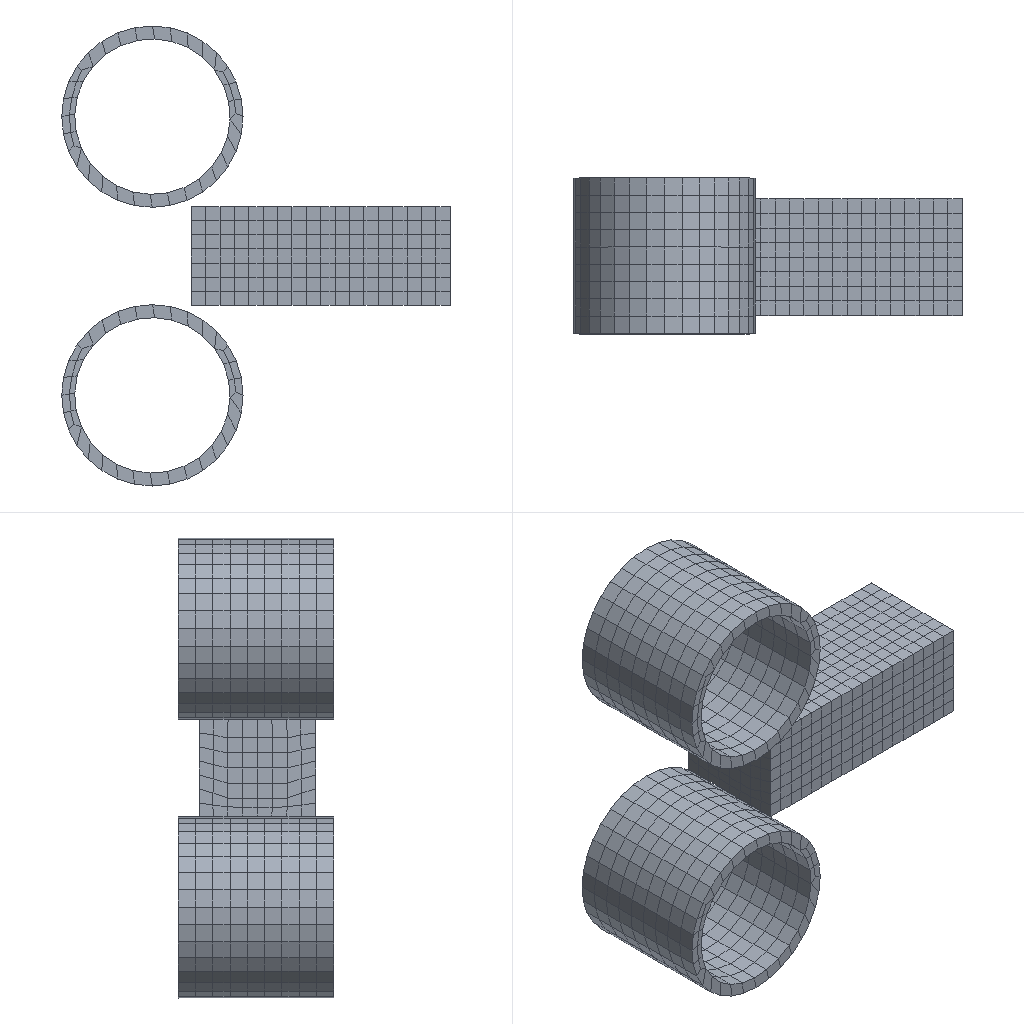Simulation study | abaqus
Set-up summary:
category,name,step,type,value,unit,region
solver,abaqus
solver,version,,,Abaqus/Explicit 2020
units,not stated in the deck,,not stated
analysis,deck,,dynamic temperature-displacement,dynamic temperature-displacement
load_step,Step-1,Step-1,dynamic temperature-displacement
load_step,requested,,,1
mesh,nodes,,,2768
mesh,elements,,,1728
element_type,C3D8R,,solid,720
element_type,C3D8RT,,solid,1008
load,load commands in deck,,count,3
bc,support commands in deck,,count,7
material,GUNZI,,in results
material,WORK,,in results
check,setup vs results,,match,"per instance, exact: element labels, types and connectivity; labels of the nodes the elements use; coordinates not compared"
Abaqus input file, long lists of numbers shortened:
*Heading
** Job name: Job-2 Model name: Model-1-Copy
** Generated by: Abaqus/CAE 2020
*Preprint, echo=NO, model=NO, history=NO, contact=NO
**
** PARTS
**
*Part, name=Part-1
*Node
      1,        1000.,  -108.96,   306.04
      2,        1000.,  -341.04,   306.04
** (1366 more lines like these left out)
*Element, type=C3D8RT
  1,   58,  349,  927,  247,    1,   17,  229,   28
  2,  349,  350,  928,  927,   17,   18,  230,  229
** (1006 more lines like these left out)
*Nset, nset=Set-6, generate
    1,  1368,     1
*Elset, elset=Set-6, generate
    1,  1008,     1
** Section: Section-1
*Solid Section, elset=Set-6, material=work
,
*End Part
**
*Part, name=gun
*Node
      1,   228.892,  -193.929,           0.
      2,   266.306,  -138.133,           0.
** (698 more lines like these left out)
*Element, type=C3D8R
  1, 107,  80,  81, 108,  37,  10,  11,  38
  2, 109, 108,  81,  82,  39,  38,  11,  12
** (358 more lines like these left out)
*Nset, nset=Set-3, generate
   1,  700,    1
*Elset, elset=Set-3, generate
   1,  360,    1
** Section: Section-2
*Solid Section, elset=Set-3, material=gunzi
,
*End Part
**
**
** ASSEMBLY
**
*Assembly, name=Assembly
**
*Instance, name=Part-1-1, part=Part-1
        150.,         -80.,        -728.
*End Instance
**
*Instance, name=gun-1, part=gun
          0.,           0.,           0.
          0.,           0.,           0., 1.,           0.,           0., 90.
*End Instance
**
*Instance, name=gun-1-lin-2-1, part=gun
          0.,           0.,       -1076.
          0.,           0.,       -1076., 1.,           0.,       -1076., 90.
*End Instance
**
*Node
      1,           0.,        -300.,       -1076.
*Node
      2,           0.,        -300., 1.83697018e-14
*Nset, nset=Set-3, instance=Part-1-1, generate
    1,  1368,     1
*Elset, elset=Set-3, instance=Part-1-1, generate
    1,  1008,     1
*Nset, nset=Set-4, instance=Part-1-1, generate
    1,  1368,     1
*Elset, elset=Set-4, instance=Part-1-1, generate
    1,  1008,     1
*Nset, nset=Set-9
 1, 2
*Nset, nset=Set-11, instance=Part-1-1, generate
    1,  1368,     1
*Elset, elset=Set-11, instance=Part-1-1, generate
    1,  1008,     1
*Nset, nset=Set-12, instance=Part-1-1, generate
    1,  1368,     1
*Elset, elset=Set-12, instance=Part-1-1, generate
    1,  1008,     1
*Nset, nset=Set-13, instance=Part-1-1
   1,   2,   3,   4,  17,  18,  19,  20,  21,  22,  23,  24,  25,  26,  27,  28
 229, 230, 231, 232, 233, 234, 235, 236, 237
*Elset, elset=Set-13, instance=Part-1-1, generate
  1,  16,   1
*Nset, nset=Set-14, instance=Part-1-1
   5,   6,   7,   8,   9,  10,  11,  12,  13,  14,  15,  16,  29,  30,  31,  32
  33,  34,  35,  36,  37,  38,  39,  40, 116, 117, 118, 119, 120, 121, 129, 130
** (21 more lines like these left out)
*Elset, elset=Set-14, instance=Part-1-1
  273,  274,  275,  276,  277,  278,  279,  280,  281,  282,  283,  284,  285,  286,  287,  288
  289,  298,  300,  301,  306,  308,  309,  310,  311,  312,  319,  321,  323,  325,  329,  338
** (17 more lines like these left out)
*Nset, nset=Set-15, instance=Part-1-1
   5,   6,   7,   8,  29,  30,  31,  32,  33,  34,  35,  36,  37,  38,  39,  40
 238, 239, 240, 241, 242, 243, 244, 245, 246
*Elset, elset=Set-15, instance=Part-1-1, generate
 273,  288,    1
*Nset, nset=Set-16, instance=Part-1-1
   5,   6,   7,   8,  29,  30,  31,  32,  33,  34,  35,  36,  37,  38,  39,  40
 238, 239, 240, 241, 242, 243, 244, 245, 246
*Elset, elset=Set-16, instance=Part-1-1, generate
 273,  288,    1
*Nset, nset=Set-17, instance=gun-1, generate
   1,  700,    1
*Nset, nset=Set-17, instance=gun-1-lin-2-1, generate
   1,  700,    1
*Elset, elset=Set-17, instance=gun-1, generate
   1,  360,    1
*Elset, elset=Set-17, instance=gun-1-lin-2-1, generate
   1,  360,    1
*Nset, nset=b_Set-5, instance=gun-1-lin-2-1, generate
   1,  700,    1
*Elset, elset=b_Set-5, instance=gun-1-lin-2-1, generate
   1,  360,    1
*Nset, nset=b_Set-7, instance=gun-1, generate
   1,  700,    1
*Elset, elset=b_Set-7, instance=gun-1, generate
   1,  360,    1
*Nset, nset=_PickedSet44, internal
 1,
*Nset, nset=_PickedSet46, internal
 2,
*Elset, elset=_Surf-18_S6, internal, instance=Part-1-1
  294,  300,  301,  303,  306,  308,  309,  310,  311,  312,  313,  314,  316,  322,  323,  328
  334,  340,  341,  343,  346,  348,  349,  350,  351,  352,  353,  354,  356,  362,  363,  368
** (16 more lines like these left out)
*Elset, elset=_Surf-18_S4, internal, instance=Part-1-1
  307,  318,  325,  347,  358,  365,  387,  398,  405,  427,  438,  445,  467,  478,  485,  507
  518,  525,  547,  558,  565,  587,  598,  605,  627,  638,  645,  667,  678,  685,  707,  718
** (2 more lines like these left out)
*Elset, elset=_Surf-18_S2, internal, instance=Part-1-1, generate
  969,  1008,     1
*Elset, elset=_Surf-18_S1, internal, instance=Part-1-1, generate
 273,  288,    1
*Elset, elset=_Surf-18_S3, internal, instance=Part-1-1
  289,  295,  297,  298,  301,  306,  319,  321,  329,  335,  337,  338,  341,  346,  359,  361
  369,  375,  377,  378,  381,  386,  399,  401,  409,  415,  417,  418,  421,  426,  439,  441
** (7 more lines like these left out)
*Elset, elset=_Surf-18_S5, internal, instance=Part-1-1
  308,  323,  327,  348,  363,  367,  388,  403,  407,  428,  443,  447,  468,  483,  487,  508
  523,  527,  548,  563,  567,  588,  603,  607,  628,  643,  647,  668,  683,  687,  708,  723
** (2 more lines like these left out)
*Surface, type=ELEMENT, name=Surf-18
_Surf-18_S6, S6
_Surf-18_S4, S4
_Surf-18_S2, S2
_Surf-18_S1, S1
_Surf-18_S3, S3
_Surf-18_S5, S5
*Elset, elset=_Surf-19_S6, internal, instance=Part-1-1
  294,  300,  301,  303,  306,  308,  309,  310,  311,  312,  313,  314,  316,  322,  323,  328
  334,  340,  341,  343,  346,  348,  349,  350,  351,  352,  353,  354,  356,  362,  363,  368
** (16 more lines like these left out)
*Elset, elset=_Surf-19_S4, internal, instance=Part-1-1
  307,  318,  325,  347,  358,  365,  387,  398,  405,  427,  438,  445,  467,  478,  485,  507
  518,  525,  547,  558,  565,  587,  598,  605,  627,  638,  645,  667,  678,  685,  707,  718
** (2 more lines like these left out)
*Elset, elset=_Surf-19_S2, internal, instance=Part-1-1, generate
  969,  1008,     1
*Elset, elset=_Surf-19_S1, internal, instance=Part-1-1, generate
 273,  288,    1
*Elset, elset=_Surf-19_S3, internal, instance=Part-1-1
  289,  295,  297,  298,  301,  306,  319,  321,  329,  335,  337,  338,  341,  346,  359,  361
  369,  375,  377,  378,  381,  386,  399,  401,  409,  415,  417,  418,  421,  426,  439,  441
** (7 more lines like these left out)
*Elset, elset=_Surf-19_S5, internal, instance=Part-1-1
  308,  323,  327,  348,  363,  367,  388,  403,  407,  428,  443,  447,  468,  483,  487,  508
  523,  527,  548,  563,  567,  588,  603,  607,  628,  643,  647,  668,  683,  687,  708,  723
** (2 more lines like these left out)
*Surface, type=ELEMENT, name=Surf-19
_Surf-19_S6, S6
_Surf-19_S4, S4
_Surf-19_S2, S2
_Surf-19_S1, S1
_Surf-19_S3, S3
_Surf-19_S5, S5
*Elset, elset=_Surf-20_S6, internal, instance=Part-1-1
  294,  300,  301,  303,  306,  308,  309,  310,  311,  312,  313,  314,  316,  322,  323,  328
  334,  340,  341,  343,  346,  348,  349,  350,  351,  352,  353,  354,  356,  362,  363,  368
** (16 more lines like these left out)
*Elset, elset=_Surf-20_S4, internal, instance=Part-1-1
  307,  318,  325,  347,  358,  365,  387,  398,  405,  427,  438,  445,  467,  478,  485,  507
  518,  525,  547,  558,  565,  587,  598,  605,  627,  638,  645,  667,  678,  685,  707,  718
** (2 more lines like these left out)
*Elset, elset=_Surf-20_S2, internal, instance=Part-1-1, generate
  969,  1008,     1
*Elset, elset=_Surf-20_S1, internal, instance=Part-1-1, generate
 273,  288,    1
*Elset, elset=_Surf-20_S3, internal, instance=Part-1-1
  289,  295,  297,  298,  301,  306,  319,  321,  329,  335,  337,  338,  341,  346,  359,  361
  369,  375,  377,  378,  381,  386,  399,  401,  409,  415,  417,  418,  421,  426,  439,  441
** (7 more lines like these left out)
*Elset, elset=_Surf-20_S5, internal, instance=Part-1-1
  308,  323,  327,  348,  363,  367,  388,  403,  407,  428,  443,  447,  468,  483,  487,  508
  523,  527,  548,  563,  567,  588,  603,  607,  628,  643,  647,  668,  683,  687,  708,  723
** (2 more lines like these left out)
*Surface, type=ELEMENT, name=Surf-20
_Surf-20_S6, S6
_Surf-20_S4, S4
_Surf-20_S2, S2
_Surf-20_S1, S1
_Surf-20_S3, S3
_Surf-20_S5, S5
*Elset, elset=_Surf-21_S6, internal, instance=Part-1-1
  294,  300,  301,  303,  306,  308,  309,  310,  311,  312,  313,  314,  316,  322,  323,  328
  334,  340,  341,  343,  346,  348,  349,  350,  351,  352,  353,  354,  356,  362,  363,  368
** (16 more lines like these left out)
*Elset, elset=_Surf-21_S4, internal, instance=Part-1-1
  307,  318,  325,  347,  358,  365,  387,  398,  405,  427,  438,  445,  467,  478,  485,  507
  518,  525,  547,  558,  565,  587,  598,  605,  627,  638,  645,  667,  678,  685,  707,  718
** (2 more lines like these left out)
*Elset, elset=_Surf-21_S2, internal, instance=Part-1-1, generate
  969,  1008,     1
*Elset, elset=_Surf-21_S1, internal, instance=Part-1-1, generate
 273,  288,    1
*Elset, elset=_Surf-21_S3, internal, instance=Part-1-1
  289,  295,  297,  298,  301,  306,  319,  321,  329,  335,  337,  338,  341,  346,  359,  361
  369,  375,  377,  378,  381,  386,  399,  401,  409,  415,  417,  418,  421,  426,  439,  441
** (7 more lines like these left out)
*Elset, elset=_Surf-21_S5, internal, instance=Part-1-1
  308,  323,  327,  348,  363,  367,  388,  403,  407,  428,  443,  447,  468,  483,  487,  508
  523,  527,  548,  563,  567,  588,  603,  607,  628,  643,  647,  668,  683,  687,  708,  723
** (2 more lines like these left out)
*Surface, type=ELEMENT, name=Surf-21
_Surf-21_S6, S6
_Surf-21_S4, S4
_Surf-21_S2, S2
_Surf-21_S1, S1
_Surf-21_S3, S3
_Surf-21_S5, S5
*Elset, elset=_Surf-22_S6, internal, instance=Part-1-1
  294,  300,  301,  303,  306,  308,  309,  310,  311,  312,  313,  314,  316,  322,  323,  328
  334,  340,  341,  343,  346,  348,  349,  350,  351,  352,  353,  354,  356,  362,  363,  368
** (16 more lines like these left out)
*Elset, elset=_Surf-22_S4, internal, instance=Part-1-1
  307,  318,  325,  347,  358,  365,  387,  398,  405,  427,  438,  445,  467,  478,  485,  507
  518,  525,  547,  558,  565,  587,  598,  605,  627,  638,  645,  667,  678,  685,  707,  718
** (2 more lines like these left out)
*Elset, elset=_Surf-22_S2, internal, instance=Part-1-1, generate
  969,  1008,     1
*Elset, elset=_Surf-22_S1, internal, instance=Part-1-1, generate
 273,  288,    1
*Elset, elset=_Surf-22_S3, internal, instance=Part-1-1
  289,  295,  297,  298,  301,  306,  319,  321,  329,  335,  337,  338,  341,  346,  359,  361
  369,  375,  377,  378,  381,  386,  399,  401,  409,  415,  417,  418,  421,  426,  439,  441
** (7 more lines like these left out)
*Elset, elset=_Surf-22_S5, internal, instance=Part-1-1
  308,  323,  327,  348,  363,  367,  388,  403,  407,  428,  443,  447,  468,  483,  487,  508
  523,  527,  548,  563,  567,  588,  603,  607,  628,  643,  647,  668,  683,  687,  708,  723
** (2 more lines like these left out)
*Surface, type=ELEMENT, name=Surf-22
_Surf-22_S6, S6
_Surf-22_S4, S4
_Surf-22_S2, S2
_Surf-22_S1, S1
_Surf-22_S3, S3
_Surf-22_S5, S5
*Elset, elset=_Surf-23_S6, internal, instance=Part-1-1
  294,  300,  301,  303,  306,  308,  309,  310,  311,  312,  313,  314,  316,  322,  323,  328
  334,  340,  341,  343,  346,  348,  349,  350,  351,  352,  353,  354,  356,  362,  363,  368
** (16 more lines like these left out)
*Elset, elset=_Surf-23_S4, internal, instance=Part-1-1
  307,  318,  325,  347,  358,  365,  387,  398,  405,  427,  438,  445,  467,  478,  485,  507
  518,  525,  547,  558,  565,  587,  598,  605,  627,  638,  645,  667,  678,  685,  707,  718
** (2 more lines like these left out)
*Elset, elset=_Surf-23_S2, internal, instance=Part-1-1, generate
  969,  1008,     1
*Elset, elset=_Surf-23_S1, internal, instance=Part-1-1, generate
 273,  288,    1
*Elset, elset=_Surf-23_S3, internal, instance=Part-1-1
  289,  295,  297,  298,  301,  306,  319,  321,  329,  335,  337,  338,  341,  346,  359,  361
  369,  375,  377,  378,  381,  386,  399,  401,  409,  415,  417,  418,  421,  426,  439,  441
** (7 more lines like these left out)
*Elset, elset=_Surf-23_S5, internal, instance=Part-1-1
  308,  323,  327,  348,  363,  367,  388,  403,  407,  428,  443,  447,  468,  483,  487,  508
  523,  527,  548,  563,  567,  588,  603,  607,  628,  643,  647,  668,  683,  687,  708,  723
** (2 more lines like these left out)
*Surface, type=ELEMENT, name=Surf-23
_Surf-23_S6, S6
_Surf-23_S4, S4
_Surf-23_S2, S2
_Surf-23_S1, S1
_Surf-23_S3, S3
_Surf-23_S5, S5
*Elset, elset=_Surf-24_S6, internal, instance=Part-1-1
  294,  300,  301,  303,  306,  308,  309,  310,  311,  312,  313,  314,  316,  322,  323,  328
  334,  340,  341,  343,  346,  348,  349,  350,  351,  352,  353,  354,  356,  362,  363,  368
** (16 more lines like these left out)
*Elset, elset=_Surf-24_S4, internal, instance=Part-1-1
  307,  318,  325,  347,  358,  365,  387,  398,  405,  427,  438,  445,  467,  478,  485,  507
  518,  525,  547,  558,  565,  587,  598,  605,  627,  638,  645,  667,  678,  685,  707,  718
** (2 more lines like these left out)
*Elset, elset=_Surf-24_S2, internal, instance=Part-1-1, generate
  969,  1008,     1
*Elset, elset=_Surf-24_S1, internal, instance=Part-1-1, generate
 273,  288,    1
*Elset, elset=_Surf-24_S3, internal, instance=Part-1-1
  289,  295,  297,  298,  301,  306,  319,  321,  329,  335,  337,  338,  341,  346,  359,  361
  369,  375,  377,  378,  381,  386,  399,  401,  409,  415,  417,  418,  421,  426,  439,  441
** (7 more lines like these left out)
*Elset, elset=_Surf-24_S5, internal, instance=Part-1-1
  308,  323,  327,  348,  363,  367,  388,  403,  407,  428,  443,  447,  468,  483,  487,  508
  523,  527,  548,  563,  567,  588,  603,  607,  628,  643,  647,  668,  683,  687,  708,  723
** (2 more lines like these left out)
*Surface, type=ELEMENT, name=Surf-24
_Surf-24_S6, S6
_Surf-24_S4, S4
_Surf-24_S2, S2
_Surf-24_S1, S1
_Surf-24_S3, S3
_Surf-24_S5, S5
*Elset, elset=_Surf-25_S6, internal, instance=Part-1-1
  294,  300,  301,  303,  306,  308,  309,  310,  311,  312,  313,  314,  316,  322,  323,  328
  334,  340,  341,  343,  346,  348,  349,  350,  351,  352,  353,  354,  356,  362,  363,  368
** (16 more lines like these left out)
*Elset, elset=_Surf-25_S4, internal, instance=Part-1-1
  307,  318,  325,  347,  358,  365,  387,  398,  405,  427,  438,  445,  467,  478,  485,  507
  518,  525,  547,  558,  565,  587,  598,  605,  627,  638,  645,  667,  678,  685,  707,  718
** (2 more lines like these left out)
*Elset, elset=_Surf-25_S2, internal, instance=Part-1-1, generate
  969,  1008,     1
*Elset, elset=_Surf-25_S1, internal, instance=Part-1-1, generate
 273,  288,    1
*Elset, elset=_Surf-25_S3, internal, instance=Part-1-1
  289,  295,  297,  298,  301,  306,  319,  321,  329,  335,  337,  338,  341,  346,  359,  361
  369,  375,  377,  378,  381,  386,  399,  401,  409,  415,  417,  418,  421,  426,  439,  441
** (7 more lines like these left out)
*Elset, elset=_Surf-25_S5, internal, instance=Part-1-1
  308,  323,  327,  348,  363,  367,  388,  403,  407,  428,  443,  447,  468,  483,  487,  508
  523,  527,  548,  563,  567,  588,  603,  607,  628,  643,  647,  668,  683,  687,  708,  723
** (2 more lines like these left out)
*Surface, type=ELEMENT, name=Surf-25
_Surf-25_S6, S6
_Surf-25_S4, S4
_Surf-25_S2, S2
_Surf-25_S1, S1
_Surf-25_S3, S3
_Surf-25_S5, S5
*Elset, elset=_Surf-26_S6, internal, instance=Part-1-1
  294,  300,  301,  303,  306,  308,  309,  310,  311,  312,  313,  314,  316,  322,  323,  328
  334,  340,  341,  343,  346,  348,  349,  350,  351,  352,  353,  354,  356,  362,  363,  368
** (16 more lines like these left out)
*Elset, elset=_Surf-26_S4, internal, instance=Part-1-1
  307,  318,  325,  347,  358,  365,  387,  398,  405,  427,  438,  445,  467,  478,  485,  507
  518,  525,  547,  558,  565,  587,  598,  605,  627,  638,  645,  667,  678,  685,  707,  718
** (2 more lines like these left out)
*Elset, elset=_Surf-26_S2, internal, instance=Part-1-1, generate
  969,  1008,     1
*Elset, elset=_Surf-26_S1, internal, instance=Part-1-1, generate
 273,  288,    1
*Elset, elset=_Surf-26_S3, internal, instance=Part-1-1
  289,  295,  297,  298,  301,  306,  319,  321,  329,  335,  337,  338,  341,  346,  359,  361
  369,  375,  377,  378,  381,  386,  399,  401,  409,  415,  417,  418,  421,  426,  439,  441
** (7 more lines like these left out)
*Elset, elset=_Surf-26_S5, internal, instance=Part-1-1
  308,  323,  327,  348,  363,  367,  388,  403,  407,  428,  443,  447,  468,  483,  487,  508
  523,  527,  548,  563,  567,  588,  603,  607,  628,  643,  647,  668,  683,  687,  708,  723
** (2 more lines like these left out)
*Surface, type=ELEMENT, name=Surf-26
_Surf-26_S6, S6
_Surf-26_S4, S4
_Surf-26_S2, S2
_Surf-26_S1, S1
_Surf-26_S3, S3
_Surf-26_S5, S5
*Elset, elset=_Surf-27_S6, internal, instance=Part-1-1
  294,  300,  301,  303,  306,  308,  309,  310,  311,  312,  313,  314,  316,  322,  323,  328
  334,  340,  341,  343,  346,  348,  349,  350,  351,  352,  353,  354,  356,  362,  363,  368
** (16 more lines like these left out)
*Elset, elset=_Surf-27_S4, internal, instance=Part-1-1
  307,  318,  325,  347,  358,  365,  387,  398,  405,  427,  438,  445,  467,  478,  485,  507
  518,  525,  547,  558,  565,  587,  598,  605,  627,  638,  645,  667,  678,  685,  707,  718
** (2 more lines like these left out)
*Elset, elset=_Surf-27_S2, internal, instance=Part-1-1, generate
  969,  1008,     1
*Elset, elset=_Surf-27_S1, internal, instance=Part-1-1, generate
 273,  288,    1
*Elset, elset=_Surf-27_S3, internal, instance=Part-1-1
  289,  295,  297,  298,  301,  306,  319,  321,  329,  335,  337,  338,  341,  346,  359,  361
  369,  375,  377,  378,  381,  386,  399,  401,  409,  415,  417,  418,  421,  426,  439,  441
** (7 more lines like these left out)
*Elset, elset=_Surf-27_S5, internal, instance=Part-1-1
  308,  323,  327,  348,  363,  367,  388,  403,  407,  428,  443,  447,  468,  483,  487,  508
  523,  527,  548,  563,  567,  588,  603,  607,  628,  643,  647,  668,  683,  687,  708,  723
** (2 more lines like these left out)
*Surface, type=ELEMENT, name=Surf-27
_Surf-27_S6, S6
_Surf-27_S4, S4
_Surf-27_S2, S2
_Surf-27_S1, S1
_Surf-27_S3, S3
_Surf-27_S5, S5
*Elset, elset=_Surf-32_S6, internal, instance=Part-1-1
  294,  300,  301,  303,  306,  308,  309,  310,  311,  312,  313,  314,  316,  322,  323,  328
  334,  340,  341,  343,  346,  348,  349,  350,  351,  352,  353,  354,  356,  362,  363,  368
** (16 more lines like these left out)
*Elset, elset=_Surf-32_S4, internal, instance=Part-1-1
  307,  318,  325,  347,  358,  365,  387,  398,  405,  427,  438,  445,  467,  478,  485,  507
  518,  525,  547,  558,  565,  587,  598,  605,  627,  638,  645,  667,  678,  685,  707,  718
** (2 more lines like these left out)
*Elset, elset=_Surf-32_S2, internal, instance=Part-1-1, generate
  969,  1008,     1
*Elset, elset=_Surf-32_S1, internal, instance=Part-1-1, generate
 273,  288,    1
*Elset, elset=_Surf-32_S3, internal, instance=Part-1-1
  289,  295,  297,  298,  301,  306,  319,  321,  329,  335,  337,  338,  341,  346,  359,  361
  369,  375,  377,  378,  381,  386,  399,  401,  409,  415,  417,  418,  421,  426,  439,  441
** (7 more lines like these left out)
*Elset, elset=_Surf-32_S5, internal, instance=Part-1-1
  308,  323,  327,  348,  363,  367,  388,  403,  407,  428,  443,  447,  468,  483,  487,  508
  523,  527,  548,  563,  567,  588,  603,  607,  628,  643,  647,  668,  683,  687,  708,  723
** (2 more lines like these left out)
*Surface, type=ELEMENT, name=Surf-32
_Surf-32_S6, S6
_Surf-32_S4, S4
_Surf-32_S2, S2
_Surf-32_S1, S1
_Surf-32_S3, S3
_Surf-32_S5, S5
*Elset, elset=_Surf-33_S6, internal, instance=Part-1-1
  294,  300,  301,  303,  306,  308,  309,  310,  311,  312,  313,  314,  316,  322,  323,  328
  334,  340,  341,  343,  346,  348,  349,  350,  351,  352,  353,  354,  356,  362,  363,  368
** (16 more lines like these left out)
*Elset, elset=_Surf-33_S4, internal, instance=Part-1-1
  307,  318,  325,  347,  358,  365,  387,  398,  405,  427,  438,  445,  467,  478,  485,  507
  518,  525,  547,  558,  565,  587,  598,  605,  627,  638,  645,  667,  678,  685,  707,  718
** (2 more lines like these left out)
*Elset, elset=_Surf-33_S2, internal, instance=Part-1-1, generate
  969,  1008,     1
*Elset, elset=_Surf-33_S1, internal, instance=Part-1-1, generate
 273,  288,    1
*Elset, elset=_Surf-33_S3, internal, instance=Part-1-1
  289,  295,  297,  298,  301,  306,  319,  321,  329,  335,  337,  338,  341,  346,  359,  361
  369,  375,  377,  378,  381,  386,  399,  401,  409,  415,  417,  418,  421,  426,  439,  441
** (7 more lines like these left out)
*Elset, elset=_Surf-33_S5, internal, instance=Part-1-1
  308,  323,  327,  348,  363,  367,  388,  403,  407,  428,  443,  447,  468,  483,  487,  508
  523,  527,  548,  563,  567,  588,  603,  607,  628,  643,  647,  668,  683,  687,  708,  723
** (2 more lines like these left out)
*Surface, type=ELEMENT, name=Surf-33
_Surf-33_S6, S6
_Surf-33_S4, S4
_Surf-33_S2, S2
_Surf-33_S1, S1
_Surf-33_S3, S3
_Surf-33_S5, S5
*Elset, elset=_Surf-34_S2, internal, instance=Part-1-1
    1,    2,    3,    4,    5,    6,    7,    8,    9,   10,   11,   12,   13,   14,   15,   16
  969,  970,  971,  972,  973,  974,  975,  976,  977,  978,  979,  980,  981,  982,  983,  984
** (2 more lines like these left out)
*Elset, elset=_Surf-34_S1, internal, instance=Part-1-1, generate
 273,  328,    1
*Elset, elset=_Surf-34_S6, internal, instance=Part-1-1
  294,  300,  301,  303,  306,  308,  309,  310,  311,  312,  313,  314,  316,  322,  323,  328
  334,  340,  341,  343,  346,  348,  349,  350,  351,  352,  353,  354,  356,  362,  363,  368
** (16 more lines like these left out)
*Elset, elset=_Surf-34_S4, internal, instance=Part-1-1
  307,  318,  325,  347,  358,  365,  387,  398,  405,  427,  438,  445,  467,  478,  485,  507
  518,  525,  547,  558,  565,  587,  598,  605,  627,  638,  645,  667,  678,  685,  707,  718
** (2 more lines like these left out)
*Elset, elset=_Surf-34_S3, internal, instance=Part-1-1
  289,  295,  297,  298,  301,  306,  319,  321,  329,  335,  337,  338,  341,  346,  359,  361
  369,  375,  377,  378,  381,  386,  399,  401,  409,  415,  417,  418,  421,  426,  439,  441
** (7 more lines like these left out)
*Elset, elset=_Surf-34_S5, internal, instance=Part-1-1
  308,  323,  327,  348,  363,  367,  388,  403,  407,  428,  443,  447,  468,  483,  487,  508
  523,  527,  548,  563,  567,  588,  603,  607,  628,  643,  647,  668,  683,  687,  708,  723
** (2 more lines like these left out)
*Surface, type=ELEMENT, name=Surf-34
_Surf-34_S2, S2
_Surf-34_S1, S1
_Surf-34_S6, S6
_Surf-34_S4, S4
_Surf-34_S3, S3
_Surf-34_S5, S5
*Elset, elset=_Surf-35_S2, internal, instance=Part-1-1
    1,    2,    3,    4,    5,    6,    7,    8,    9,   10,   11,   12,   13,   14,   15,   16
  969,  970,  971,  972,  973,  974,  975,  976,  977,  978,  979,  980,  981,  982,  983,  984
** (2 more lines like these left out)
*Elset, elset=_Surf-35_S1, internal, instance=Part-1-1, generate
 273,  328,    1
*Elset, elset=_Surf-35_S6, internal, instance=Part-1-1
  294,  300,  301,  303,  306,  308,  309,  310,  311,  312,  313,  314,  316,  322,  323,  328
  334,  340,  341,  343,  346,  348,  349,  350,  351,  352,  353,  354,  356,  362,  363,  368
** (16 more lines like these left out)
*Elset, elset=_Surf-35_S4, internal, instance=Part-1-1
  307,  318,  325,  347,  358,  365,  387,  398,  405,  427,  438,  445,  467,  478,  485,  507
  518,  525,  547,  558,  565,  587,  598,  605,  627,  638,  645,  667,  678,  685,  707,  718
** (2 more lines like these left out)
*Elset, elset=_Surf-35_S3, internal, instance=Part-1-1
  289,  295,  297,  298,  301,  306,  319,  321,  329,  335,  337,  338,  341,  346,  359,  361
  369,  375,  377,  378,  381,  386,  399,  401,  409,  415,  417,  418,  421,  426,  439,  441
** (7 more lines like these left out)
*Elset, elset=_Surf-35_S5, internal, instance=Part-1-1
  308,  323,  327,  348,  363,  367,  388,  403,  407,  428,  443,  447,  468,  483,  487,  508
  523,  527,  548,  563,  567,  588,  603,  607,  628,  643,  647,  668,  683,  687,  708,  723
** (2 more lines like these left out)
*Surface, type=ELEMENT, name=Surf-35
_Surf-35_S2, S2
_Surf-35_S1, S1
_Surf-35_S6, S6
_Surf-35_S4, S4
_Surf-35_S3, S3
_Surf-35_S5, S5
*Elset, elset=_m_Surf-28_S6, internal, instance=gun-1-lin-2-1
   1,   5,   7,   9,  10,  11,  12,  13,  14,  15,  18,  36,  38,  41,  45,  47
  49,  50,  51,  52,  53,  54,  55,  58,  76,  78,  81,  85,  87,  89,  90,  91
** (6 more lines like these left out)
*Elset, elset=_m_Surf-28_S3, internal, instance=gun-1-lin-2-1
   2,   3,  21,  26,  27,  35,  42,  43,  61,  66,  67,  75,  82,  83, 101, 106
 107, 115, 122, 123, 141, 146, 147, 155, 162, 163, 181, 186, 187, 195, 202, 203
** (2 more lines like these left out)
*Elset, elset=_m_Surf-28_S5, internal, instance=gun-1-lin-2-1
   4,  22,  23,  24,  25,  34,  44,  62,  63,  64,  65,  74,  84, 102, 103, 104
 105, 114, 124, 142, 143, 144, 145, 154, 164, 182, 183, 184, 185, 194, 204, 222
** (2 more lines like these left out)
*Elset, elset=_m_Surf-28_S4, internal, instance=gun-1-lin-2-1
   6,   8,  16,  17,  28,  29,  39,  46,  48,  56,  57,  68,  69,  79,  86,  88
  96,  97, 108, 109, 119, 126, 128, 136, 137, 148, 149, 159, 166, 168, 176, 177
** (2 more lines like these left out)
*Surface, type=ELEMENT, name=m_Surf-28
_m_Surf-28_S6, S6
_m_Surf-28_S3, S3
_m_Surf-28_S4, S4
_m_Surf-28_S5, S5
*Elset, elset=_m_Surf-30_S6, internal, instance=gun-1
   1,   5,   7,   9,  10,  11,  12,  13,  14,  15,  18,  36,  38,  41,  45,  47
  49,  50,  51,  52,  53,  54,  55,  58,  76,  78,  81,  85,  87,  89,  90,  91
** (6 more lines like these left out)
*Elset, elset=_m_Surf-30_S3, internal, instance=gun-1
   2,   3,  21,  26,  27,  35,  42,  43,  61,  66,  67,  75,  82,  83, 101, 106
 107, 115, 122, 123, 141, 146, 147, 155, 162, 163, 181, 186, 187, 195, 202, 203
** (2 more lines like these left out)
*Elset, elset=_m_Surf-30_S5, internal, instance=gun-1
   4,  22,  23,  24,  25,  34,  44,  62,  63,  64,  65,  74,  84, 102, 103, 104
 105, 114, 124, 142, 143, 144, 145, 154, 164, 182, 183, 184, 185, 194, 204, 222
** (2 more lines like these left out)
*Elset, elset=_m_Surf-30_S4, internal, instance=gun-1
   6,   8,  16,  17,  28,  29,  39,  46,  48,  56,  57,  68,  69,  79,  86,  88
  96,  97, 108, 109, 119, 126, 128, 136, 137, 148, 149, 159, 166, 168, 176, 177
** (2 more lines like these left out)
*Surface, type=ELEMENT, name=m_Surf-30
_m_Surf-30_S6, S6
_m_Surf-30_S3, S3
_m_Surf-30_S4, S4
_m_Surf-30_S5, S5
*Elset, elset=_s_Surf-28_S6, internal, instance=Part-1-1
  300,  301,  303,  306,  308,  309,  310,  311,  312,  313,  314,  316,  323,  328,  340,  341
  343,  346,  348,  349,  350,  351,  352,  353,  354,  356,  363,  368,  380,  381,  383,  386
** (14 more lines like these left out)
*Elset, elset=_s_Surf-28_S4, internal, instance=Part-1-1
  318,  325,  358,  365,  398,  405,  438,  445,  478,  485,  518,  525,  558,  565,  598,  605
  638,  645,  678,  685,  718,  725,  758,  765,  798,  805,  838,  845,  878,  885,  918,  925
** (1 more lines like these left out)
*Elset, elset=_s_Surf-28_S2, internal, instance=Part-1-1, generate
  969,  1008,     1
*Elset, elset=_s_Surf-28_S1, internal, instance=Part-1-1, generate
 273,  288,    1
*Elset, elset=_s_Surf-28_S3, internal, instance=Part-1-1
  289,  298,  301,  319,  321,  329,  338,  341,  359,  361,  369,  378,  381,  399,  401,  409
  418,  421,  439,  441,  449,  458,  461,  479,  481,  489,  498,  501,  519,  521,  529,  538
** (4 more lines like these left out)
*Elset, elset=_s_Surf-28_S5, internal, instance=Part-1-1, generate
 308,  988,   40
*Surface, type=ELEMENT, name=s_Surf-28
_s_Surf-28_S6, S6
_s_Surf-28_S4, S4
_s_Surf-28_S2, S2
_s_Surf-28_S1, S1
_s_Surf-28_S3, S3
_s_Surf-28_S5, S5
*Elset, elset=_s_Surf-30_S6, internal, instance=Part-1-1
  294,  300,  301,  306,  308,  309,  310,  311,  312,  322,  323,  334,  340,  341,  346,  348
  349,  350,  351,  352,  362,  363,  374,  380,  381,  386,  388,  389,  390,  391,  392,  402
** (11 more lines like these left out)
*Elset, elset=_s_Surf-30_S4, internal, instance=Part-1-1
  307,  325,  347,  365,  387,  405,  427,  445,  467,  485,  507,  525,  547,  565,  587,  605
  627,  645,  667,  685,  707,  725,  747,  765,  787,  805,  827,  845,  867,  885,  907,  925
** (1 more lines like these left out)
*Elset, elset=_s_Surf-30_S2, internal, instance=Part-1-1, generate
  969,  1008,     1
*Elset, elset=_s_Surf-30_S1, internal, instance=Part-1-1, generate
 273,  288,    1
*Elset, elset=_s_Surf-30_S3, internal, instance=Part-1-1
  289,  295,  297,  298,  306,  319,  321,  329,  335,  337,  338,  346,  359,  361,  369,  375
  377,  378,  386,  399,  401,  409,  415,  417,  418,  426,  439,  441,  449,  455,  457,  458
** (6 more lines like these left out)
*Elset, elset=_s_Surf-30_S5, internal, instance=Part-1-1
  323,  327,  363,  367,  403,  407,  443,  447,  483,  487,  523,  527,  563,  567,  603,  607
  643,  647,  683,  687,  723,  727,  763,  767,  803,  807,  843,  847,  883,  887,  923,  927
** (1 more lines like these left out)
*Surface, type=ELEMENT, name=s_Surf-30
_s_Surf-30_S6, S6
_s_Surf-30_S4, S4
_s_Surf-30_S2, S2
_s_Surf-30_S1, S1
_s_Surf-30_S3, S3
_s_Surf-30_S5, S5
** Constraint: Constraint-1
*Rigid Body, ref node=_PickedSet44, elset=b_Set-5, position=CENTER OF MASS
** Constraint: Constraint-2
*Rigid Body, ref node=_PickedSet46, elset=b_Set-7, position=CENTER OF MASS
*End Assembly
**
** MATERIALS
**
*Material, name=gunzi
*Density
 7.8e-09,
*Elastic
210000., 0.3
*Material, name=work
*Conductivity
    20.7,  30.
 21.702, 344.
 22.662, 444.
 23.622, 544.
 24.582, 644.
 25.542, 744.
 26.502, 844.
 27.462, 944.
 28.422,1044.
 29.382,1144.
 30.342,1244.
 31.302,1344.
*Density
 7.8e-09,
*Elastic
 175000., 0.3274,    100.
 175000., 0.3274,    200.
 175000., 0.3274,    300.
 175000., 0.3274,    400.
 175000., 0.3274,    499.
 172500., 0.3274,    500.
 137470., 0.3274,    600.
 102439., 0.3356,    700.
 67408.5, 0.3438,    800.
 32728.3, 0.352,    899.
  32378., 0.3521,    900.
  20000.,  0.3603,   1000.
  14542., 0.3685,   1100.
  12896., 0.3768,   1200.
  11954., 0.385,   1300.
 10961.7, 0.3886,   1344.
 10925.5, 0.4187,   1345.
*Expansion
 1.18276e-05, 100.
 1.28536e-05, 200.
 1.37901e-05, 300.
 1.46372e-05, 400.
 1.54581e-05, 499.
 1.61496e-05, 500.
 1.67178e-05, 600.
 1.69072e-05, 700.
 1.72861e-05, 800.
 2.23733e-05, 899.
  2.3457e-05, 900.
 2.86125e-05,1000.
 3.17815e-05,1100.
 3.44199e-05,1200.
 3.59217e-05,1300.
 3.70582e-05,1344.
 3.70582e-05,1345.
*Plastic
160.,  0., 30.
190., 0.1, 30.
200., 0.2, 30.
210., 0.3, 30.
212., 0.4, 30.
214., 0.5, 30.
215., 0.6, 30.
*Specific Heat
 5.73229e+08,  30.
 5.82749e+08, 344.
 5.92269e+08, 444.
 6.01789e+08, 544.
 6.11309e+08, 644.
 6.20829e+08, 744.
 6.30349e+08, 844.
 6.39869e+08, 944.
 6.49389e+08,1044.
 6.58909e+08,1144.
 6.68429e+08,1244.
 6.77949e+08,1344.
**
** INTERACTION PROPERTIES
**
*Surface Interaction, name=IntProp-1
*Friction
 0.5,
*Surface Behavior, pressure-overclosure=HARD
*Gap Heat Generation
1., 0.5
**
** PHYSICAL CONSTANTS
**
*Physical Constants, absolute zero=-273., stefan boltzmann=5.67e-08
**
** BOUNDARY CONDITIONS
**
** Name: BC-1 Type: 对称/反对称/完全固定
*Boundary
Set-9, ENCASTRE
**
** PREDEFINED FIELDS
**
** Name: Predefined Field-1   Type: Temperature
*Initial Conditions, type=TEMPERATURE, file=D:\__________\_____\_____.___________________
** Name: Predefined Field-2   Type: Temperature
*Initial Conditions, type=TEMPERATURE
Set-17, 30.
** ----------------------------------------------------------------
**
** STEP: Step-1
**
*Step, name=Step-1, nlgeom=YES
*Dynamic Temperature-displacement, Explicit
, 10.
*Bulk Viscosity
0.06, 1.2
** Mass Scaling: Semi-Automatic
**               Whole Model
*Fixed Mass Scaling, factor=500.
**
** BOUNDARY CONDITIONS
**
** Name: BC-4 Type: 速度/角速度
*Boundary, type=VELOCITY
Set-16, 1, 1, -110.
Set-16, 2, 2
Set-16, 3, 3
Set-16, 4, 4
Set-16, 5, 5
Set-16, 6, 6
**
** INTERACTIONS
**
** Interaction: Int-1
*Contact Pair, interaction=IntProp-1, mechanical constraint=KINEMATIC, cpset=Int-1
m_Surf-28, s_Surf-28
** Interaction: Int-2
*Contact Pair, interaction=IntProp-1, mechanical constraint=KINEMATIC, cpset=Int-2
m_Surf-30, s_Surf-30
** Interaction: Int-3
*Sfilm
Surf-34, F, 30., 0.1
** Interaction: Int-4
*Sradiate
Surf-35, R, 30., 0.5
**
** OUTPUT REQUESTS
**
*Restart, write, number interval=1, time marks=NO
**
** FIELD OUTPUT: F-Output-1
**
*Output, field, number interval=50
*Node Output
A, NT, RF, RFL, RM, RT, U, V
*Element Output, directions=YES
E, HFL, LE, MISES, MISESMAX, PE, PEEQ, PEMAG, PEVAVG, S, SVAVG, TEMP, VEEQ
**
** HISTORY OUTPUT: H-Output-1
**
*Output, history, variable=PRESELECT
*End Step
Results summary:
result,step,Step-1,completed,increments=73681 time=10.0/10.0
result,analysis,,,"dynamic temperature-displacement, explict"
result,last_loadstep,,,1
result,primary field,,,"U, NT11"
result,reaction total,,FX,-512301.102,model units
result,reaction total,,FY,9657.562,model units
result,reaction total,,FZ,-128848.19,model units